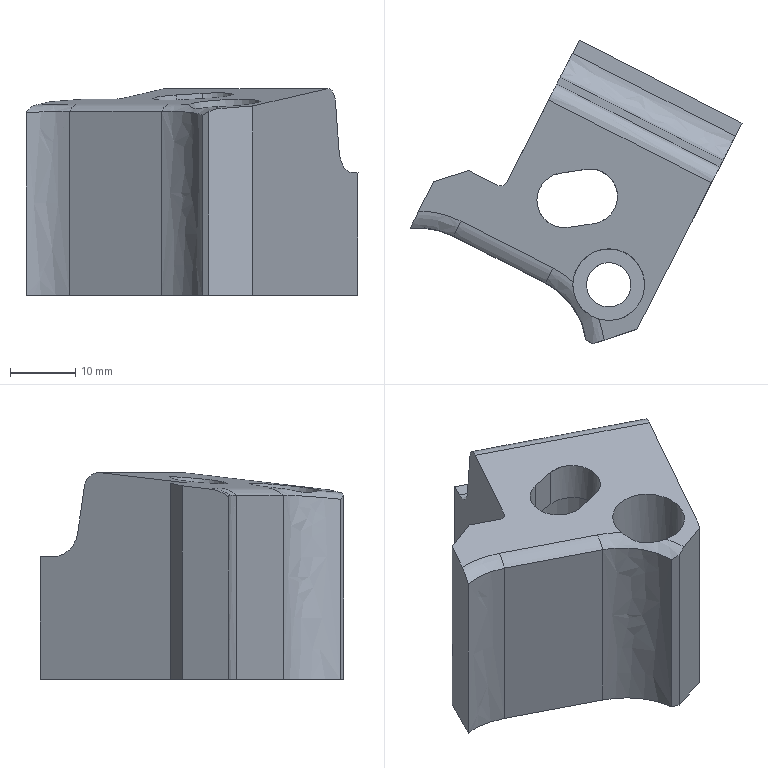Part | STEP file | gslz 2016.10.28-13_id514_x_t | 1 solid | 32 faces | box 50.88 x 46.528 x 31.681 mm | volume 25870 mm3 | plane 14 | spline 8 | cylinder 6 | other 4 | commonest cylinder face diameters 8.4 x2 2 x1 6.8 x1 11 x1 14 x1